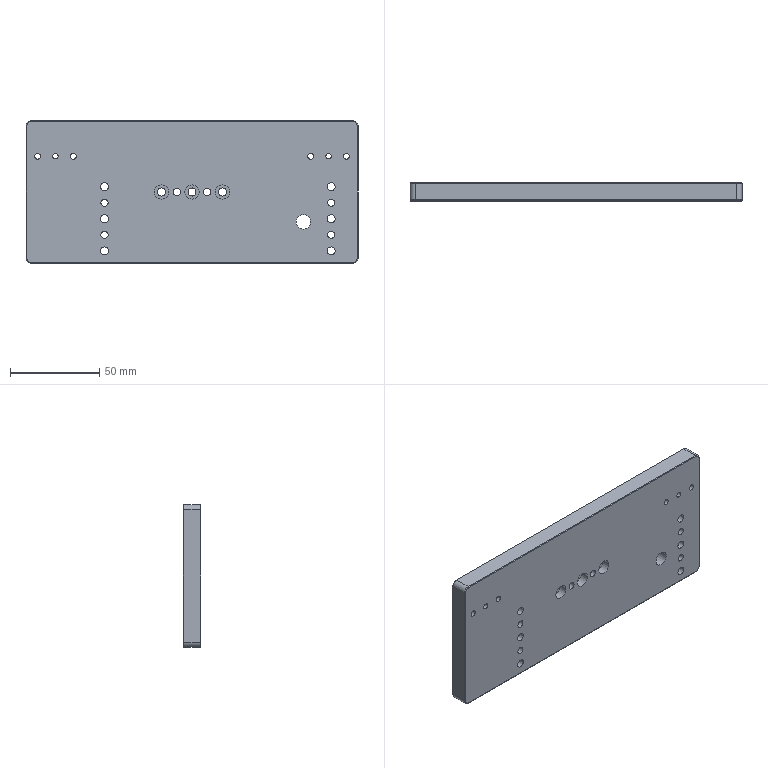CAM job | NX | 3+2 milling, drilling | part box 186 x 10 x 80 mm | stock box 191 x 12 x 85 mm
Tools:
number,name,description,diameter,corner_radius,flute_length,length,flutes
3,D3,平底铣刀-粗,3.0,0.0,20.0,75.0,2
4,D4,平底铣刀-粗,4.0,0.0,25.0,75.0,2
9,D10,平底铣刀-粗,10.0,0.0,35.0,75.0,2
17,D3-J,平底铣刀-精,3.0,0.0,50.0,75.0,2
10,D10-J,平底铣刀-精,10.0,0.0,35.0,75.0,2
1,D80R0.8飞刀,圆鼻刀-粗,80.0,0.8,50.0,75.0,2
1,D80R0.8飞刀-J,圆鼻刀-精,80.0,0.8,50.0,75.0,2
2,D6倒角刀,倒角刀,6.0,0.0,3.0,25.0,2
21,M4X0.7,丝锥,3.3,0.0,35.0,50.0,2
23,D4铰刀,Drilling Tool,4.0,0.0,75.0,100.0,6
18,ZT3,钻头,3.0,0.0,35.0,50.0,2
11,ZT4.5,钻头,4.5,0.0,35.0,50.0,2
17,ZT8,钻头,8.0,0.0,35.0,50.0,2
13,钻头3.3,Twist Drill 3.3 mm,3.3,0.0,35.0,35.008,2
19,ZT3.9,Drilling Tool,3.9,0.0,35.0,50.0,2
Operations:
program,operation,operation_type,tool,method,geometry_group,spindle_rpm,surface_speed,feed_per_tooth,feed_cut,feed_plunge,cut_length_mm,path_length_mm,cut_time_min,machine_time_min
B,底壁铣飞面开粗_COPY,VolumeBased25DMillingOperation,D80R0.8飞刀,分层开粗-切深K-步距G,W-B,2800.0,703.696,0.5357,3000.0,100.0,2325.702,2442.566,0.7752,0.7869
B,底壁铣飞面精光_COPY,VolumeBased25DMillingOperation,D80R0.8飞刀-J,侧刃精光-切深K-步距G,W-B,4000.0,1005.28,0.125,1000.0,100.0,580.841,616.841,0.5808,0.5844
B,铣沉头_2,CylinderMilling,D4,METHOD,W-B,6000.0,75.398,0.15,1800.0,100.0,1128.193,1610.993,0.6268,0.6751
B,铣沉头_1,CylinderMilling,D3,METHOD,W-B,6000.0,56.549,0.0917,1100.0,100.0,373.444,617.844,0.3395,0.3639
B,铣孔_2,CylinderMilling,D3-J,METHOD,W-B,6000.0,75.398,0.05,600.0,100.0,129.922,642.122,0.2165,0.2678
B,钻倒角_4,Operation,D6倒角刀,METHOD,W-B,7000.0,131.947,0.0357,500.0,0.0,20.8,264.081,0.0416,0.0659
B,钻倒角_5,Operation,D6倒角刀,METHOD,W-B,7000.0,131.947,0.0357,500.0,0.0,31.2,282.034,0.0624,0.0875
B,钻倒角_6,Operation,D6倒角刀,METHOD,W-B,7000.0,131.947,0.0357,500.0,0.0,16.35,113.225,0.0327,0.0424
B,铣倒角_4,PlanarMilling,D6倒角刀,METHOD,W-B,7000.0,131.947,0.0429,600.0,100.0,36.041,272.428,0.0601,0.0837
B,铣倒角_5,PlanarMilling,D6倒角刀,METHOD,W-B,7000.0,131.947,0.0429,600.0,100.0,122.676,578.025,0.2045,0.25
B,铣倒角_6,PlanarMilling,D6倒角刀,METHOD,W-B,7000.0,131.947,0.0429,600.0,100.0,23.915,65.715,0.0399,0.044
B,底壁铣倒角_COPY_1,VolumeBased25DMillingOperation,D6倒角刀,爬面_倒角-切深0-步距G,W-B,6500.0,122.519,0.1154,1500.0,100.0,538.27,577.67,0.3588,0.3628
B,底壁铣精光侧面-中-选底面_COPY,VolumeBased25DMillingOperation,D3-J,侧刃精光-切深K-步距G,W-B,8000.0,75.398,0.0187,300.0,100.0,45.166,265.879,0.1506,0.1726
A,顶面,FaceMilling,D80R0.8飞刀,侧刃精光-切深K-步距G,W-A,5000.0,1256.637,0.1,1000.0,100.0,599.333,635.333,0.5993,0.6029
A,外形粗_2,VolumeBased25DMillingOperation,D10,METHOD,W-A,8000.0,251.327,0.3125,5000.0,80.0,8384.914,8433.514,1.677,1.682
A,打点-深0.8,Operation,D6倒角刀,NONE,W-A,8000.0,150.796,0.0312,500.0,90.0,39.6,447.457,0.0792,0.12
A,通孔-6-8,Operation,ZT8,NONE,W-A,2500.0,62.832,0.06,300.0,90.0,15.403,70.807,0.0513,0.0569
A,通孔-5-6,Operation,ZT4.5,NONE,W-A,3000.0,42.411,0.0417,250.0,90.0,87.0,418.115,0.348,0.3811
A,沉头孔-钻孔0段,Operation,ZT4.5,NONE,W-A,2800.0,39.584,0.0357,200.0,90.0,43.056,162.17,0.2153,0.2272
A,通孔-M4螺纹底孔,Operation,钻头3.3,NONE,W-A,3000.0,31.102,0.05,300.0,90.0,67.966,351.985,0.2266,0.255
A,通孔-精孔3.0预钻,Operation,ZT3,NONE,W-A,3200.0,29.154,0.0312,200.0,90.0,28.0,250.003,0.14,0.1622
A,通孔-精孔4.0预钻,Operation,ZT3.9,NONE,W-A,3000.0,36.757,0.0417,250.0,90.0,90.755,390.315,0.363,0.393
A,铣孔开粗D4_1,CylinderMilling,D4,NONE,W-A,8000.0,100.531,0.075,1200.0,100.0,662.754,829.054,0.5523,0.5689
A,铣孔精光D4_1,CylinderMilling,D4,精光步距切深关,W-A,8000.0,100.531,0.0312,500.0,100.0,97.761,264.061,0.1955,0.2122
A,钻倒角_1,Operation,D6倒角刀,METHOD,W-A,8000.0,150.796,0.0312,500.0,0.0,9.6,215.229,0.0192,0.0398
A,钻倒角_2,Operation,D6倒角刀,METHOD,W-A,8000.0,150.796,0.0312,500.0,0.0,20.8,264.081,0.0416,0.0659
A,钻倒角_3,Operation,D6倒角刀,METHOD,W-A,8000.0,150.796,0.0312,500.0,0.0,31.8,283.234,0.0636,0.0887
A,铣倒角_1,PlanarMilling,D6倒角刀,METHOD,W-A,8000.0,150.796,0.0312,500.0,100.0,104.118,550.351,0.2082,0.2529
A,铣倒角_2,PlanarMilling,D6倒角刀,NONE,W-A,8000.0,150.796,0.0312,500.0,100.0,101.903,248.623,0.2038,0.2185
A,铣倒角_3,PlanarMilling,D6倒角刀,METHOD,W-A,8000.0,150.796,0.05,800.0,100.0,32.589,73.589,0.0407,0.0448
A,底壁铣倒角_COPY,VolumeBased25DMillingOperation,D6倒角刀,爬面_倒角-切深0-步距G,W-A,6500.0,122.519,0.1154,1500.0,100.0,538.27,577.67,0.3588,0.3628
A,通孔-攻牙M4,Operation,M4X0.7,METHOD,W-A,600.0,6.22,0.0006,0.7,90.0,56.0,328.054,80.0,80.027
A,铰孔_2,Operation,D4铰刀,METHOD,W-A,500.0,6.283,0.0167,50.0,0.0,72.0,352.805,1.44,1.468
A,外形半精_2,VolumeBased25DMillingOperation,D10-J,METHOD,W-A,8000.0,251.327,0.0625,1000.0,100.0,563.251,622.452,0.5633,0.5692